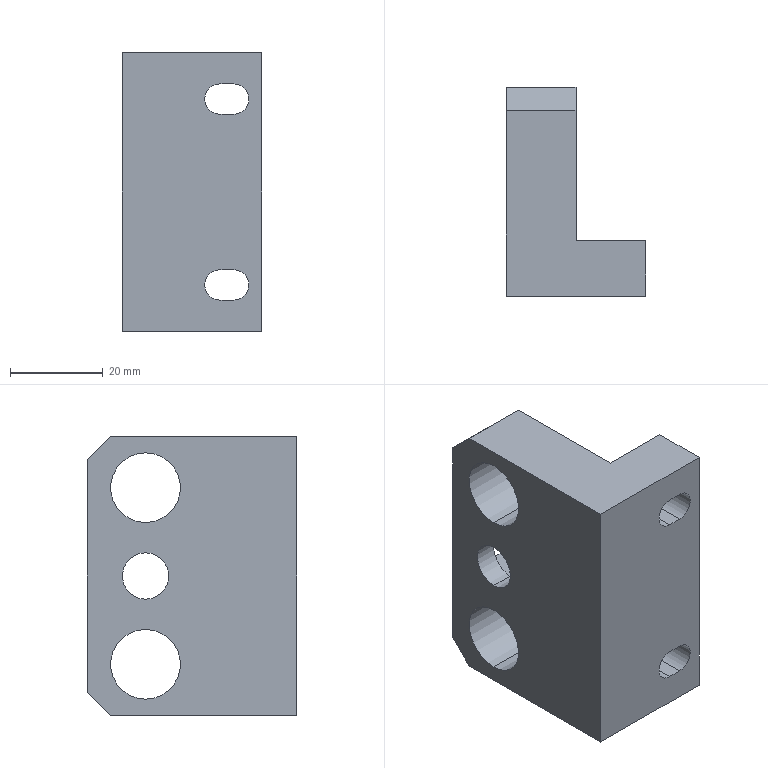Part | STEP file | defective part push material cylinder seat | 1 solid | 30 faces | box 30 x 45 x 60 mm | volume 39635 mm3 | plane 18 | cylinder 12 | commonest cylinder face diameters 6.5 x4 15 x4 8 x2 10 x2